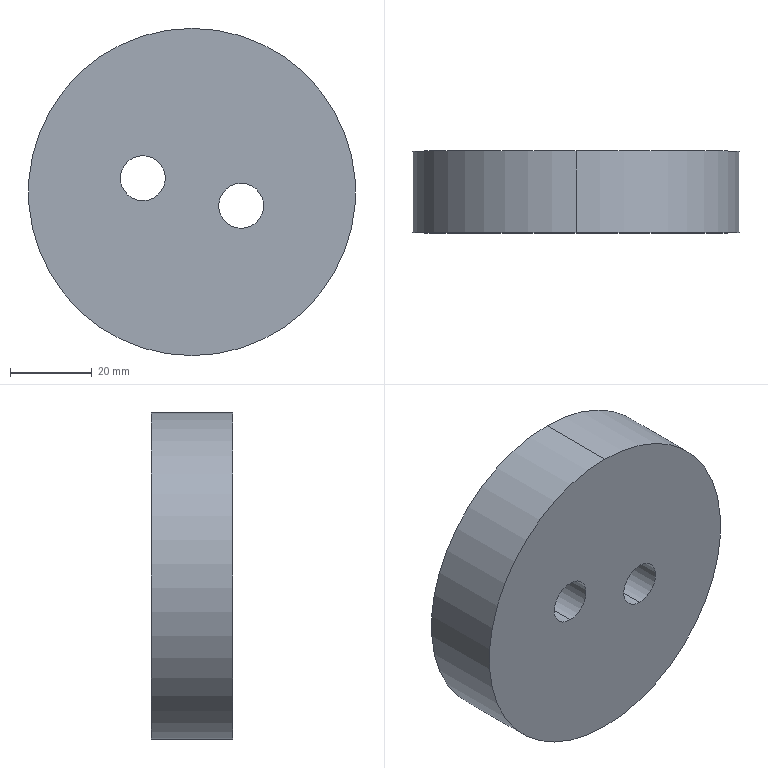Part | SolidWorks | features 3DProfileFeature 1, Extrusion 1, HoleWzd 1 | 1 solid | 14 faces | box 80 x 20 x 80 mm | volume 93222 mm3 | cylinder 10 | plane 4 | commonest cylinder face diameters 11 x4 18 x4 80 x2
STEP:
#1=CARTESIAN_POINT('',(-12.034,9.,-5.62));
#2=VERTEX_POINT('',#1);
#3=CARTESIAN_POINT('',(-12.034,9.,12.38));
#4=VERTEX_POINT('',#3);
#5=CARTESIAN_POINT('',(-12.034,9.,3.38));
#6=DIRECTION('',(0.,1.,0.));
#7=DIRECTION('',(0.,0.,1.));
#8=AXIS2_PLACEMENT_3D('',#5,#6,#7);
#9=CIRCLE('',#8,9.);
#10=EDGE_CURVE('',#2,#4,#9,.T.);
#11=ORIENTED_EDGE('',*,*,#10,.F.);
#12=CARTESIAN_POINT('',(-12.034,20.,-5.62));
#13=VERTEX_POINT('',#12);
#14=CARTESIAN_POINT('',(-12.034,20.,-5.62));
#15=DIRECTION('',(0.,1.,0.));
#16=VECTOR('',#15,1000.);
#17=LINE('',#14,#16);
#18=EDGE_CURVE('',#2,#13,#17,.T.);
#19=ORIENTED_EDGE('',*,*,#18,.T.);
#20=CARTESIAN_POINT('',(-12.034,20.,12.38));
#21=VERTEX_POINT('',#20);
#22=CARTESIAN_POINT('',(-12.034,20.,3.38));
#23=DIRECTION('',(0.,1.,0.));
#24=DIRECTION('',(0.,0.,1.));
#25=AXIS2_PLACEMENT_3D('',#22,#23,#24);
#26=CIRCLE('',#25,9.);
#27=EDGE_CURVE('',#13,#21,#26,.T.);
#28=ORIENTED_EDGE('',*,*,#27,.T.);
#29=CARTESIAN_POINT('',(-12.034,20.,12.38));
#30=DIRECTION('',(0.,1.,0.));
#31=VECTOR('',#30,1000.);
#32=LINE('',#29,#31);
#33=EDGE_CURVE('',#4,#21,#32,.T.);
#34=ORIENTED_EDGE('',*,*,#33,.F.);
#35=EDGE_LOOP('',(#11,#19,#28,#34));
#36=FACE_OUTER_BOUND('',#35,.T.);
#37=CARTESIAN_POINT('',(-12.034,20.,3.38));
#38=DIRECTION('',(0.,1.,0.));
#39=DIRECTION('',(0.,0.,1.));
#40=AXIS2_PLACEMENT_3D('',#37,#38,#39);
#41=CYLINDRICAL_SURFACE('',#40,9.);
#42=ADVANCED_FACE('',(#36),#41,.F.);
#43=CARTESIAN_POINT('',(-12.034,0.,-2.12));
#44=VERTEX_POINT('',#43);
#45=CARTESIAN_POINT('',(-12.034,0.,8.88));
#46=VERTEX_POINT('',#45);
#47=CARTESIAN_POINT('',(-12.034,0.,3.38));
#48=DIRECTION('',(0.,1.,0.));
#49=DIRECTION('',(0.,0.,1.));
#50=AXIS2_PLACEMENT_3D('',#47,#48,#49);
#51=CIRCLE('',#50,5.5);
#52=EDGE_CURVE('',#44,#46,#51,.T.);
#53=ORIENTED_EDGE('',*,*,#52,.F.);
#54=CARTESIAN_POINT('',(-12.034,9.,-2.12));
#55=VERTEX_POINT('',#54);
#56=CARTESIAN_POINT('',(-12.034,20.,-2.12));
#57=DIRECTION('',(0.,1.,0.));
#58=VECTOR('',#57,1000.);
#59=LINE('',#56,#58);
#60=EDGE_CURVE('',#44,#55,#59,.T.);
#61=ORIENTED_EDGE('',*,*,#60,.T.);
#62=CARTESIAN_POINT('',(-12.034,9.,8.88));
#63=VERTEX_POINT('',#62);
#64=CARTESIAN_POINT('',(-12.034,9.,3.38));
#65=DIRECTION('',(0.,1.,0.));
#66=DIRECTION('',(0.,0.,1.));
#67=AXIS2_PLACEMENT_3D('',#64,#65,#66);
#68=CIRCLE('',#67,5.5);
#69=EDGE_CURVE('',#55,#63,#68,.T.);
#70=ORIENTED_EDGE('',*,*,#69,.T.);
#71=CARTESIAN_POINT('',(-12.034,20.,8.88));
#72=DIRECTION('',(0.,1.,0.));
#73=VECTOR('',#72,1000.);
#74=LINE('',#71,#73);
#75=EDGE_CURVE('',#46,#63,#74,.T.);
#76=ORIENTED_EDGE('',*,*,#75,.F.);
#77=EDGE_LOOP('',(#53,#61,#70,#76));
#78=FACE_OUTER_BOUND('',#77,.T.);
#79=CARTESIAN_POINT('',(-12.034,20.,3.38));
#80=DIRECTION('',(0.,1.,0.));
#81=DIRECTION('',(0.,0.,1.));
#82=AXIS2_PLACEMENT_3D('',#79,#80,#81);
#83=CYLINDRICAL_SURFACE('',#82,5.5);
#84=ADVANCED_FACE('',(#78),#83,.F.);
#85=CARTESIAN_POINT('',(12.034,9.,-12.38));
#86=VERTEX_POINT('',#85);
#87=CARTESIAN_POINT('',(12.034,9.,5.62));
#88=VERTEX_POINT('',#87);
#89=CARTESIAN_POINT('',(12.034,9.,-3.38));
#90=DIRECTION('',(0.,1.,0.));
#91=DIRECTION('',(0.,0.,1.));
#92=AXIS2_PLACEMENT_3D('',#89,#90,#91);
#93=CIRCLE('',#92,9.);
#94=EDGE_CURVE('',#86,#88,#93,.T.);
#95=ORIENTED_EDGE('',*,*,#94,.F.);
#96=CARTESIAN_POINT('',(12.034,20.,-12.38));
#97=VERTEX_POINT('',#96);
#98=CARTESIAN_POINT('',(12.034,20.,-12.38));
#99=DIRECTION('',(0.,1.,0.));
#100=VECTOR('',#99,1000.);
#101=LINE('',#98,#100);
#102=EDGE_CURVE('',#86,#97,#101,.T.);
#103=ORIENTED_EDGE('',*,*,#102,.T.);
#104=CARTESIAN_POINT('',(12.034,20.,5.62));
#105=VERTEX_POINT('',#104);
#106=CARTESIAN_POINT('',(12.034,20.,-3.38));
#107=DIRECTION('',(0.,1.,0.));
#108=DIRECTION('',(0.,0.,1.));
#109=AXIS2_PLACEMENT_3D('',#106,#107,#108);
#110=CIRCLE('',#109,9.);
#111=EDGE_CURVE('',#97,#105,#110,.T.);
#112=ORIENTED_EDGE('',*,*,#111,.T.);
#113=CARTESIAN_POINT('',(12.034,20.,5.62));
#114=DIRECTION('',(0.,1.,0.));
#115=VECTOR('',#114,1000.);
#116=LINE('',#113,#115);
#117=EDGE_CURVE('',#88,#105,#116,.T.);
#118=ORIENTED_EDGE('',*,*,#117,.F.);
#119=EDGE_LOOP('',(#95,#103,#112,#118));
#120=FACE_OUTER_BOUND('',#119,.T.);
#121=CARTESIAN_POINT('',(12.034,20.,-3.38));
#122=DIRECTION('',(0.,1.,0.));
#123=DIRECTION('',(0.,0.,1.));
#124=AXIS2_PLACEMENT_3D('',#121,#122,#123);
#125=CYLINDRICAL_SURFACE('',#124,9.);
#126=ADVANCED_FACE('',(#120),#125,.F.);
#127=CARTESIAN_POINT('',(12.034,0.,-8.88));
#128=VERTEX_POINT('',#127);
#129=CARTESIAN_POINT('',(12.034,0.,2.12));
#130=VERTEX_POINT('',#129);
#131=CARTESIAN_POINT('',(12.034,0.,-3.38));
#132=DIRECTION('',(0.,1.,0.));
#133=DIRECTION('',(0.,0.,1.));
#134=AXIS2_PLACEMENT_3D('',#131,#132,#133);
#135=CIRCLE('',#134,5.5);
#136=EDGE_CURVE('',#128,#130,#135,.T.);
#137=ORIENTED_EDGE('',*,*,#136,.F.);
#138=CARTESIAN_POINT('',(12.034,9.,-8.88));
#139=VERTEX_POINT('',#138);
#140=CARTESIAN_POINT('',(12.034,20.,-8.88));
#141=DIRECTION('',(0.,1.,0.));
#142=VECTOR('',#141,1000.);
#143=LINE('',#140,#142);
#144=EDGE_CURVE('',#128,#139,#143,.T.);
#145=ORIENTED_EDGE('',*,*,#144,.T.);
#146=CARTESIAN_POINT('',(12.034,9.,2.12));
#147=VERTEX_POINT('',#146);
#148=CARTESIAN_POINT('',(12.034,9.,-3.38));
#149=DIRECTION('',(0.,1.,0.));
#150=DIRECTION('',(0.,0.,1.));
#151=AXIS2_PLACEMENT_3D('',#148,#149,#150);
#152=CIRCLE('',#151,5.5);
#153=EDGE_CURVE('',#139,#147,#152,.T.);
#154=ORIENTED_EDGE('',*,*,#153,.T.);
#155=CARTESIAN_POINT('',(12.034,20.,2.12));
#156=DIRECTION('',(0.,1.,0.));
#157=VECTOR('',#156,1000.);
#158=LINE('',#155,#157);
#159=EDGE_CURVE('',#130,#147,#158,.T.);
#160=ORIENTED_EDGE('',*,*,#159,.F.);
#161=EDGE_LOOP('',(#137,#145,#154,#160));
#162=FACE_OUTER_BOUND('',#161,.T.);
#163=CARTESIAN_POINT('',(12.034,20.,-3.38));
#164=DIRECTION('',(0.,1.,0.));
#165=DIRECTION('',(0.,0.,1.));
#166=AXIS2_PLACEMENT_3D('',#163,#164,#165);
#167=CYLINDRICAL_SURFACE('',#166,5.5);
#168=ADVANCED_FACE('',(#162),#167,.F.);
#169=CARTESIAN_POINT('',(0.,20.,40.));
#170=VERTEX_POINT('',#169);
#171=CARTESIAN_POINT('',(0.,20.,-40.));
#172=VERTEX_POINT('',#171);
#173=CARTESIAN_POINT('',(0.,20.,0.));
#174=DIRECTION('',(0.,1.,0.));
#175=DIRECTION('',(0.,0.,1.));
#176=AXIS2_PLACEMENT_3D('',#173,#174,#175);
#177=CIRCLE('',#176,40.);
#178=EDGE_CURVE('',#170,#172,#177,.T.);
#179=ORIENTED_EDGE('',*,*,#178,.F.);
#180=CARTESIAN_POINT('',(0.,0.,40.));
#181=VERTEX_POINT('',#180);
#182=CARTESIAN_POINT('',(0.,20.,40.));
#183=DIRECTION('',(0.,-1.,0.));
#184=VECTOR('',#183,1000.);
#185=LINE('',#182,#184);
#186=EDGE_CURVE('',#170,#181,#185,.T.);
#187=ORIENTED_EDGE('',*,*,#186,.T.);
#188=CARTESIAN_POINT('',(0.,0.,-40.));
#189=VERTEX_POINT('',#188);
#190=CARTESIAN_POINT('',(0.,0.,0.));
#191=DIRECTION('',(0.,1.,0.));
#192=DIRECTION('',(0.,0.,1.));
#193=AXIS2_PLACEMENT_3D('',#190,#191,#192);
#194=CIRCLE('',#193,40.);
#195=EDGE_CURVE('',#181,#189,#194,.T.);
#196=ORIENTED_EDGE('',*,*,#195,.T.);
#197=CARTESIAN_POINT('',(0.,20.,-40.));
#198=DIRECTION('',(0.,-1.,0.));
#199=VECTOR('',#198,1000.);
#200=LINE('',#197,#199);
#201=EDGE_CURVE('',#172,#189,#200,.T.);
#202=ORIENTED_EDGE('',*,*,#201,.F.);
#203=EDGE_LOOP('',(#179,#187,#196,#202));
#204=FACE_OUTER_BOUND('',#203,.T.);
#205=CARTESIAN_POINT('',(0.,20.,0.));
#206=DIRECTION('',(0.,-1.,0.));
#207=DIRECTION('',(0.,0.,-1.));
#208=AXIS2_PLACEMENT_3D('',#205,#206,#207);
#209=CYLINDRICAL_SURFACE('',#208,40.);
#210=ADVANCED_FACE('',(#204),#209,.T.);
#211=ORIENTED_EDGE('',*,*,#186,.F.);
#212=CARTESIAN_POINT('',(0.,20.,0.));
#213=DIRECTION('',(0.,1.,0.));
#214=DIRECTION('',(0.,0.,1.));
#215=AXIS2_PLACEMENT_3D('',#212,#213,#214);
#216=CIRCLE('',#215,40.);
#217=EDGE_CURVE('',#172,#170,#216,.T.);
#218=ORIENTED_EDGE('',*,*,#217,.F.);
#219=ORIENTED_EDGE('',*,*,#201,.T.);
#220=CARTESIAN_POINT('',(0.,0.,0.));
#221=DIRECTION('',(0.,1.,0.));
#222=DIRECTION('',(0.,0.,1.));
#223=AXIS2_PLACEMENT_3D('',#220,#221,#222);
#224=CIRCLE('',#223,40.);
#225=EDGE_CURVE('',#189,#181,#224,.T.);
#226=ORIENTED_EDGE('',*,*,#225,.T.);
#227=EDGE_LOOP('',(#211,#218,#219,#226));
#228=FACE_OUTER_BOUND('',#227,.T.);
#229=CARTESIAN_POINT('',(0.,20.,0.));
#230=DIRECTION('',(0.,-1.,0.));
#231=DIRECTION('',(0.,0.,-1.));
#232=AXIS2_PLACEMENT_3D('',#229,#230,#231);
#233=CYLINDRICAL_SURFACE('',#232,40.);
#234=ADVANCED_FACE('',(#228),#233,.T.);
#235=CARTESIAN_POINT('',(-12.034,20.,3.38));
#236=DIRECTION('',(0.,1.,0.));
#237=DIRECTION('',(0.,0.,1.));
#238=AXIS2_PLACEMENT_3D('',#235,#236,#237);
#239=CIRCLE('',#238,9.);
#240=EDGE_CURVE('',#21,#13,#239,.T.);
#241=ORIENTED_EDGE('',*,*,#240,.F.);
#242=ORIENTED_EDGE('',*,*,#27,.F.);
#243=EDGE_LOOP('',(#241,#242));
#244=FACE_BOUND('',#243,.T.);
#245=CARTESIAN_POINT('',(12.034,20.,-3.38));
#246=DIRECTION('',(0.,1.,0.));
#247=DIRECTION('',(0.,0.,1.));
#248=AXIS2_PLACEMENT_3D('',#245,#246,#247);
#249=CIRCLE('',#248,9.);
#250=EDGE_CURVE('',#105,#97,#249,.T.);
#251=ORIENTED_EDGE('',*,*,#250,.F.);
#252=ORIENTED_EDGE('',*,*,#111,.F.);
#253=EDGE_LOOP('',(#251,#252));
#254=FACE_BOUND('',#253,.T.);
#255=ORIENTED_EDGE('',*,*,#217,.T.);
#256=ORIENTED_EDGE('',*,*,#178,.T.);
#257=EDGE_LOOP('',(#255,#256));
#258=FACE_OUTER_BOUND('',#257,.T.);
#259=CARTESIAN_POINT('',(0.,20.,0.));
#260=DIRECTION('',(0.,1.,0.));
#261=DIRECTION('',(0.,0.,1.));
#262=AXIS2_PLACEMENT_3D('',#259,#260,#261);
#263=PLANE('',#262);
#264=ADVANCED_FACE('',(#244,#254,#258),#263,.T.);
#265=CARTESIAN_POINT('',(-12.034,0.,3.38));
#266=DIRECTION('',(0.,1.,0.));
#267=DIRECTION('',(0.,0.,1.));
#268=AXIS2_PLACEMENT_3D('',#265,#266,#267);
#269=CIRCLE('',#268,5.5);
#270=EDGE_CURVE('',#46,#44,#269,.T.);
#271=ORIENTED_EDGE('',*,*,#270,.T.);
#272=ORIENTED_EDGE('',*,*,#52,.T.);
#273=EDGE_LOOP('',(#271,#272));
#274=FACE_BOUND('',#273,.T.);
#275=CARTESIAN_POINT('',(12.034,0.,-3.38));
#276=DIRECTION('',(0.,1.,0.));
#277=DIRECTION('',(0.,0.,1.));
#278=AXIS2_PLACEMENT_3D('',#275,#276,#277);
#279=CIRCLE('',#278,5.5);
#280=EDGE_CURVE('',#130,#128,#279,.T.);
#281=ORIENTED_EDGE('',*,*,#280,.T.);
#282=ORIENTED_EDGE('',*,*,#136,.T.);
#283=EDGE_LOOP('',(#281,#282));
#284=FACE_BOUND('',#283,.T.);
#285=ORIENTED_EDGE('',*,*,#225,.F.);
#286=ORIENTED_EDGE('',*,*,#195,.F.);
#287=EDGE_LOOP('',(#285,#286));
#288=FACE_OUTER_BOUND('',#287,.T.);
#289=CARTESIAN_POINT('',(0.,0.,0.));
#290=DIRECTION('',(0.,1.,0.));
#291=DIRECTION('',(0.,0.,1.));
#292=AXIS2_PLACEMENT_3D('',#289,#290,#291);
#293=PLANE('',#292);
#294=ADVANCED_FACE('',(#274,#284,#288),#293,.F.);
#295=ORIENTED_EDGE('',*,*,#144,.F.);
#296=ORIENTED_EDGE('',*,*,#280,.F.);
#297=ORIENTED_EDGE('',*,*,#159,.T.);
#298=CARTESIAN_POINT('',(12.034,9.,-3.38));
#299=DIRECTION('',(0.,1.,0.));
#300=DIRECTION('',(0.,0.,1.));
#301=AXIS2_PLACEMENT_3D('',#298,#299,#300);
#302=CIRCLE('',#301,5.5);
#303=EDGE_CURVE('',#147,#139,#302,.T.);
#304=ORIENTED_EDGE('',*,*,#303,.T.);
#305=EDGE_LOOP('',(#295,#296,#297,#304));
#306=FACE_OUTER_BOUND('',#305,.T.);
#307=CARTESIAN_POINT('',(12.034,20.,-3.38));
#308=DIRECTION('',(0.,1.,0.));
#309=DIRECTION('',(0.,0.,1.));
#310=AXIS2_PLACEMENT_3D('',#307,#308,#309);
#311=CYLINDRICAL_SURFACE('',#310,5.5);
#312=ADVANCED_FACE('',(#306),#311,.F.);
#313=ORIENTED_EDGE('',*,*,#303,.F.);
#314=ORIENTED_EDGE('',*,*,#153,.F.);
#315=EDGE_LOOP('',(#313,#314));
#316=FACE_BOUND('',#315,.T.);
#317=CARTESIAN_POINT('',(12.034,9.,-3.38));
#318=DIRECTION('',(0.,1.,0.));
#319=DIRECTION('',(0.,0.,1.));
#320=AXIS2_PLACEMENT_3D('',#317,#318,#319);
#321=CIRCLE('',#320,9.);
#322=EDGE_CURVE('',#88,#86,#321,.T.);
#323=ORIENTED_EDGE('',*,*,#322,.T.);
#324=ORIENTED_EDGE('',*,*,#94,.T.);
#325=EDGE_LOOP('',(#323,#324));
#326=FACE_OUTER_BOUND('',#325,.T.);
#327=CARTESIAN_POINT('',(17.534,9.,-3.38));
#328=DIRECTION('',(0.,-1.,0.));
#329=DIRECTION('',(0.,0.,-1.));
#330=AXIS2_PLACEMENT_3D('',#327,#328,#329);
#331=PLANE('',#330);
#332=ADVANCED_FACE('',(#316,#326),#331,.F.);
#333=ORIENTED_EDGE('',*,*,#102,.F.);
#334=ORIENTED_EDGE('',*,*,#322,.F.);
#335=ORIENTED_EDGE('',*,*,#117,.T.);
#336=ORIENTED_EDGE('',*,*,#250,.T.);
#337=EDGE_LOOP('',(#333,#334,#335,#336));
#338=FACE_OUTER_BOUND('',#337,.T.);
#339=CARTESIAN_POINT('',(12.034,20.,-3.38));
#340=DIRECTION('',(0.,1.,0.));
#341=DIRECTION('',(0.,0.,1.));
#342=AXIS2_PLACEMENT_3D('',#339,#340,#341);
#343=CYLINDRICAL_SURFACE('',#342,9.);
#344=ADVANCED_FACE('',(#338),#343,.F.);
#345=ORIENTED_EDGE('',*,*,#60,.F.);
#346=ORIENTED_EDGE('',*,*,#270,.F.);
#347=ORIENTED_EDGE('',*,*,#75,.T.);
#348=CARTESIAN_POINT('',(-12.034,9.,3.38));
#349=DIRECTION('',(0.,1.,0.));
#350=DIRECTION('',(0.,0.,1.));
#351=AXIS2_PLACEMENT_3D('',#348,#349,#350);
#352=CIRCLE('',#351,5.5);
#353=EDGE_CURVE('',#63,#55,#352,.T.);
#354=ORIENTED_EDGE('',*,*,#353,.T.);
#355=EDGE_LOOP('',(#345,#346,#347,#354));
#356=FACE_OUTER_BOUND('',#355,.T.);
#357=CARTESIAN_POINT('',(-12.034,20.,3.38));
#358=DIRECTION('',(0.,1.,0.));
#359=DIRECTION('',(0.,0.,1.));
#360=AXIS2_PLACEMENT_3D('',#357,#358,#359);
#361=CYLINDRICAL_SURFACE('',#360,5.5);
#362=ADVANCED_FACE('',(#356),#361,.F.);
#363=ORIENTED_EDGE('',*,*,#353,.F.);
#364=ORIENTED_EDGE('',*,*,#69,.F.);
#365=EDGE_LOOP('',(#363,#364));
#366=FACE_BOUND('',#365,.T.);
#367=CARTESIAN_POINT('',(-12.034,9.,3.38));
#368=DIRECTION('',(0.,1.,0.));
#369=DIRECTION('',(0.,0.,1.));
#370=AXIS2_PLACEMENT_3D('',#367,#368,#369);
#371=CIRCLE('',#370,9.);
#372=EDGE_CURVE('',#4,#2,#371,.T.);
#373=ORIENTED_EDGE('',*,*,#372,.T.);
#374=ORIENTED_EDGE('',*,*,#10,.T.);
#375=EDGE_LOOP('',(#373,#374));
#376=FACE_OUTER_BOUND('',#375,.T.);
#377=CARTESIAN_POINT('',(-6.534,9.,3.38));
#378=DIRECTION('',(0.,-1.,0.));
#379=DIRECTION('',(0.,0.,-1.));
#380=AXIS2_PLACEMENT_3D('',#377,#378,#379);
#381=PLANE('',#380);
#382=ADVANCED_FACE('',(#366,#376),#381,.F.);
#383=ORIENTED_EDGE('',*,*,#18,.F.);
#384=ORIENTED_EDGE('',*,*,#372,.F.);
#385=ORIENTED_EDGE('',*,*,#33,.T.);
#386=ORIENTED_EDGE('',*,*,#240,.T.);
#387=EDGE_LOOP('',(#383,#384,#385,#386));
#388=FACE_OUTER_BOUND('',#387,.T.);
#389=CARTESIAN_POINT('',(-12.034,20.,3.38));
#390=DIRECTION('',(0.,1.,0.));
#391=DIRECTION('',(0.,0.,1.));
#392=AXIS2_PLACEMENT_3D('',#389,#390,#391);
#393=CYLINDRICAL_SURFACE('',#392,9.);
#394=ADVANCED_FACE('',(#388),#393,.F.);
#395=CLOSED_SHELL('',(#42,#84,#126,#168,#210,#234,#264,#294,#312,#332,#344,#362,#382,#394));
#396=MANIFOLD_SOLID_BREP('',#395);
#397=CARTESIAN_POINT('',(0.,0.,0.));
#398=DIRECTION('',(0.,0.,1.));
#399=DIRECTION('',(1.,0.,0.));
#400=AXIS2_PLACEMENT_3D('',#397,#398,#399);
#401=(LENGTH_UNIT()NAMED_UNIT(*)SI_UNIT(.MILLI.,.METRE.));
#402=UNCERTAINTY_MEASURE_WITH_UNIT(LENGTH_MEASURE(0.00001),#401,'','');
#403=(NAMED_UNIT(*)PLANE_ANGLE_UNIT()SI_UNIT($,.RADIAN.));
#404=(NAMED_UNIT(*)SI_UNIT($,.STERADIAN.)SOLID_ANGLE_UNIT());
#405=(GEOMETRIC_REPRESENTATION_CONTEXT(3)GLOBAL_UNCERTAINTY_ASSIGNED_CONTEXT((#402))GLOBAL_UNIT_ASSIGNED_CONTEXT((#401,#403,#404))REPRESENTATION_CONTEXT('',''));
#406=ADVANCED_BREP_SHAPE_REPRESENTATION('',(#396,#400),#405);